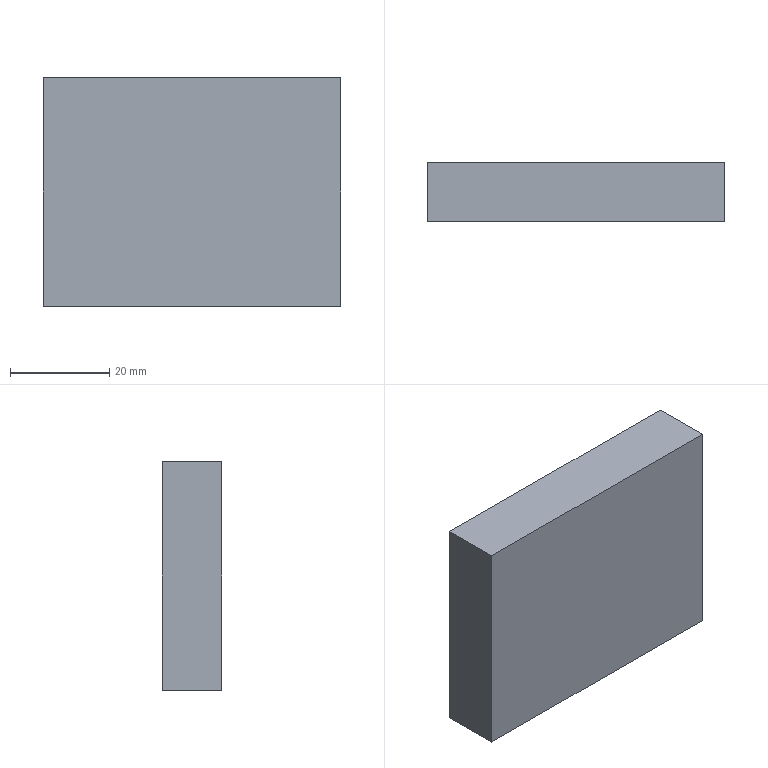Part | SolidWorks | features Extrusion 1 | 1 solid | 6 faces | box 60 x 12 x 46 mm | volume 33120 mm3 | plane 6
STEP:
#1=CARTESIAN_POINT('',(0.,0.,0.));
#2=VERTEX_POINT('',#1);
#3=CARTESIAN_POINT('',(0.,0.,46.));
#4=VERTEX_POINT('',#3);
#5=CARTESIAN_POINT('',(0.,0.,0.));
#6=DIRECTION('',(0.,0.,1.));
#7=VECTOR('',#6,1000.);
#8=LINE('',#5,#7);
#9=EDGE_CURVE('',#2,#4,#8,.T.);
#10=ORIENTED_EDGE('',*,*,#9,.T.);
#11=CARTESIAN_POINT('',(0.,12.,46.));
#12=VERTEX_POINT('',#11);
#13=CARTESIAN_POINT('',(0.,12.,46.));
#14=DIRECTION('',(0.,-1.,0.));
#15=VECTOR('',#14,1000.);
#16=LINE('',#13,#15);
#17=EDGE_CURVE('',#12,#4,#16,.T.);
#18=ORIENTED_EDGE('',*,*,#17,.F.);
#19=CARTESIAN_POINT('',(0.,12.,0.));
#20=VERTEX_POINT('',#19);
#21=CARTESIAN_POINT('',(0.,12.,0.));
#22=DIRECTION('',(0.,0.,1.));
#23=VECTOR('',#22,1000.);
#24=LINE('',#21,#23);
#25=EDGE_CURVE('',#20,#12,#24,.T.);
#26=ORIENTED_EDGE('',*,*,#25,.F.);
#27=CARTESIAN_POINT('',(0.,12.,0.));
#28=DIRECTION('',(0.,-1.,0.));
#29=VECTOR('',#28,1000.);
#30=LINE('',#27,#29);
#31=EDGE_CURVE('',#20,#2,#30,.T.);
#32=ORIENTED_EDGE('',*,*,#31,.T.);
#33=EDGE_LOOP('',(#10,#18,#26,#32));
#34=FACE_OUTER_BOUND('',#33,.T.);
#35=CARTESIAN_POINT('',(0.,12.,0.));
#36=DIRECTION('',(1.,0.,0.));
#37=DIRECTION('',(0.,0.,-1.));
#38=AXIS2_PLACEMENT_3D('',#35,#36,#37);
#39=PLANE('',#38);
#40=ADVANCED_FACE('',(#34),#39,.F.);
#41=CARTESIAN_POINT('',(60.,0.,46.));
#42=VERTEX_POINT('',#41);
#43=CARTESIAN_POINT('',(0.,0.,46.));
#44=DIRECTION('',(1.,0.,0.));
#45=VECTOR('',#44,1000.);
#46=LINE('',#43,#45);
#47=EDGE_CURVE('',#4,#42,#46,.T.);
#48=ORIENTED_EDGE('',*,*,#47,.T.);
#49=CARTESIAN_POINT('',(60.,12.,46.));
#50=VERTEX_POINT('',#49);
#51=CARTESIAN_POINT('',(60.,12.,46.));
#52=DIRECTION('',(0.,-1.,0.));
#53=VECTOR('',#52,1000.);
#54=LINE('',#51,#53);
#55=EDGE_CURVE('',#50,#42,#54,.T.);
#56=ORIENTED_EDGE('',*,*,#55,.F.);
#57=CARTESIAN_POINT('',(0.,12.,46.));
#58=DIRECTION('',(1.,0.,0.));
#59=VECTOR('',#58,1000.);
#60=LINE('',#57,#59);
#61=EDGE_CURVE('',#12,#50,#60,.T.);
#62=ORIENTED_EDGE('',*,*,#61,.F.);
#63=ORIENTED_EDGE('',*,*,#17,.T.);
#64=EDGE_LOOP('',(#48,#56,#62,#63));
#65=FACE_OUTER_BOUND('',#64,.T.);
#66=CARTESIAN_POINT('',(0.,12.,46.));
#67=DIRECTION('',(0.,0.,-1.));
#68=DIRECTION('',(-1.,0.,0.));
#69=AXIS2_PLACEMENT_3D('',#66,#67,#68);
#70=PLANE('',#69);
#71=ADVANCED_FACE('',(#65),#70,.F.);
#72=CARTESIAN_POINT('',(60.,0.,0.));
#73=VERTEX_POINT('',#72);
#74=CARTESIAN_POINT('',(60.,0.,0.));
#75=DIRECTION('',(0.,0.,-1.));
#76=VECTOR('',#75,1000.);
#77=LINE('',#74,#76);
#78=EDGE_CURVE('',#42,#73,#77,.T.);
#79=ORIENTED_EDGE('',*,*,#78,.T.);
#80=CARTESIAN_POINT('',(60.,12.,0.));
#81=VERTEX_POINT('',#80);
#82=CARTESIAN_POINT('',(60.,12.,0.));
#83=DIRECTION('',(0.,-1.,0.));
#84=VECTOR('',#83,1000.);
#85=LINE('',#82,#84);
#86=EDGE_CURVE('',#81,#73,#85,.T.);
#87=ORIENTED_EDGE('',*,*,#86,.F.);
#88=CARTESIAN_POINT('',(60.,12.,0.));
#89=DIRECTION('',(0.,0.,-1.));
#90=VECTOR('',#89,1000.);
#91=LINE('',#88,#90);
#92=EDGE_CURVE('',#50,#81,#91,.T.);
#93=ORIENTED_EDGE('',*,*,#92,.F.);
#94=ORIENTED_EDGE('',*,*,#55,.T.);
#95=EDGE_LOOP('',(#79,#87,#93,#94));
#96=FACE_OUTER_BOUND('',#95,.T.);
#97=CARTESIAN_POINT('',(60.,12.,0.));
#98=DIRECTION('',(-1.,0.,0.));
#99=DIRECTION('',(0.,0.,1.));
#100=AXIS2_PLACEMENT_3D('',#97,#98,#99);
#101=PLANE('',#100);
#102=ADVANCED_FACE('',(#96),#101,.F.);
#103=CARTESIAN_POINT('',(0.,0.,0.));
#104=DIRECTION('',(-1.,0.,0.));
#105=VECTOR('',#104,1000.);
#106=LINE('',#103,#105);
#107=EDGE_CURVE('',#73,#2,#106,.T.);
#108=ORIENTED_EDGE('',*,*,#107,.T.);
#109=ORIENTED_EDGE('',*,*,#31,.F.);
#110=CARTESIAN_POINT('',(0.,12.,0.));
#111=DIRECTION('',(-1.,0.,0.));
#112=VECTOR('',#111,1000.);
#113=LINE('',#110,#112);
#114=EDGE_CURVE('',#81,#20,#113,.T.);
#115=ORIENTED_EDGE('',*,*,#114,.F.);
#116=ORIENTED_EDGE('',*,*,#86,.T.);
#117=EDGE_LOOP('',(#108,#109,#115,#116));
#118=FACE_OUTER_BOUND('',#117,.T.);
#119=CARTESIAN_POINT('',(0.,12.,0.));
#120=DIRECTION('',(0.,0.,1.));
#121=DIRECTION('',(1.,0.,0.));
#122=AXIS2_PLACEMENT_3D('',#119,#120,#121);
#123=PLANE('',#122);
#124=ADVANCED_FACE('',(#118),#123,.F.);
#125=ORIENTED_EDGE('',*,*,#25,.T.);
#126=ORIENTED_EDGE('',*,*,#61,.T.);
#127=ORIENTED_EDGE('',*,*,#92,.T.);
#128=ORIENTED_EDGE('',*,*,#114,.T.);
#129=EDGE_LOOP('',(#125,#126,#127,#128));
#130=FACE_OUTER_BOUND('',#129,.T.);
#131=CARTESIAN_POINT('',(0.,12.,0.));
#132=DIRECTION('',(0.,1.,0.));
#133=DIRECTION('',(0.,0.,1.));
#134=AXIS2_PLACEMENT_3D('',#131,#132,#133);
#135=PLANE('',#134);
#136=ADVANCED_FACE('',(#130),#135,.T.);
#137=ORIENTED_EDGE('',*,*,#9,.F.);
#138=ORIENTED_EDGE('',*,*,#107,.F.);
#139=ORIENTED_EDGE('',*,*,#78,.F.);
#140=ORIENTED_EDGE('',*,*,#47,.F.);
#141=EDGE_LOOP('',(#137,#138,#139,#140));
#142=FACE_OUTER_BOUND('',#141,.T.);
#143=CARTESIAN_POINT('',(0.,0.,0.));
#144=DIRECTION('',(0.,1.,0.));
#145=DIRECTION('',(0.,0.,1.));
#146=AXIS2_PLACEMENT_3D('',#143,#144,#145);
#147=PLANE('',#146);
#148=ADVANCED_FACE('',(#142),#147,.F.);
#149=CLOSED_SHELL('',(#40,#71,#102,#124,#136,#148));
#150=MANIFOLD_SOLID_BREP('',#149);
#151=CARTESIAN_POINT('',(0.,0.,0.));
#152=DIRECTION('',(0.,0.,1.));
#153=DIRECTION('',(1.,0.,0.));
#154=AXIS2_PLACEMENT_3D('',#151,#152,#153);
#155=(LENGTH_UNIT()NAMED_UNIT(*)SI_UNIT(.MILLI.,.METRE.));
#156=UNCERTAINTY_MEASURE_WITH_UNIT(LENGTH_MEASURE(0.00001),#155,'','');
#157=(NAMED_UNIT(*)PLANE_ANGLE_UNIT()SI_UNIT($,.RADIAN.));
#158=(NAMED_UNIT(*)SI_UNIT($,.STERADIAN.)SOLID_ANGLE_UNIT());
#159=(GEOMETRIC_REPRESENTATION_CONTEXT(3)GLOBAL_UNCERTAINTY_ASSIGNED_CONTEXT((#156))GLOBAL_UNIT_ASSIGNED_CONTEXT((#155,#157,#158))REPRESENTATION_CONTEXT('',''));
#160=ADVANCED_BREP_SHAPE_REPRESENTATION('',(#150,#154),#159);